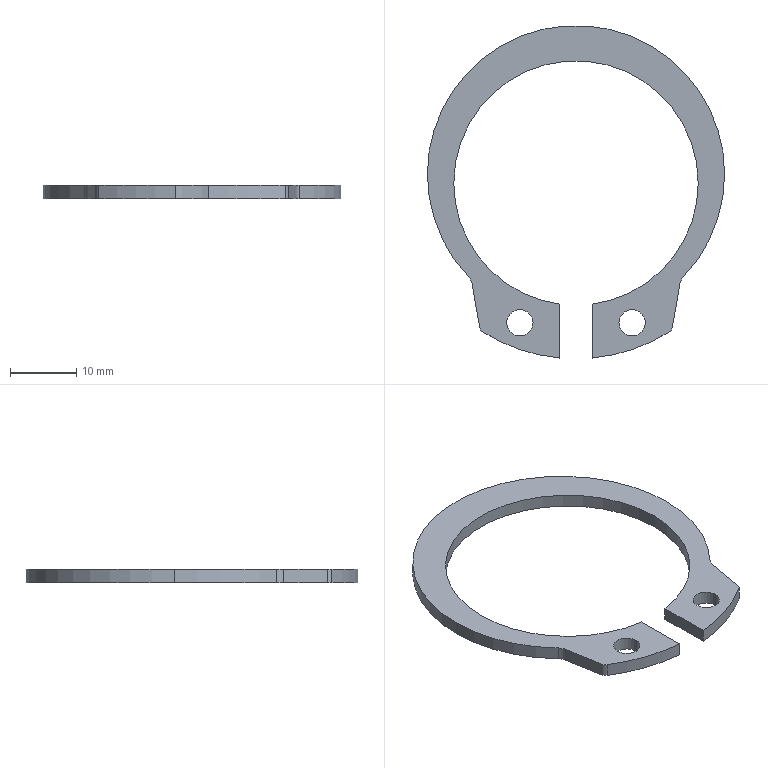Part | SolidWorks | features Extrusion 1 | 1 solid | 22 faces | box 45 x 50.322 x 2 mm | volume 1249 mm3 | cylinder 16 | plane 6 | commonest cylinder face diameters 4 x6 37 x3 45 x3 2 x2 53.2 x2
STEP:
#1=CARTESIAN_POINT('',(6.5,-22.5,2.));
#2=VERTEX_POINT('',#1);
#3=CARTESIAN_POINT('',(10.5,-22.5,2.));
#4=VERTEX_POINT('',#3);
#5=CARTESIAN_POINT('',(8.5,-22.5,2.));
#6=DIRECTION('',(0.,0.,1.));
#7=DIRECTION('',(1.,0.,0.));
#8=AXIS2_PLACEMENT_3D('',#5,#6,#7);
#9=CIRCLE('',#8,2.);
#10=EDGE_CURVE('',#2,#4,#9,.T.);
#11=ORIENTED_EDGE('',*,*,#10,.T.);
#12=CARTESIAN_POINT('',(10.5,-22.5,0.));
#13=VERTEX_POINT('',#12);
#14=CARTESIAN_POINT('',(10.5,-22.5,2.));
#15=DIRECTION('',(0.,0.,-1.));
#16=VECTOR('',#15,1000.);
#17=LINE('',#14,#16);
#18=EDGE_CURVE('',#4,#13,#17,.T.);
#19=ORIENTED_EDGE('',*,*,#18,.T.);
#20=CARTESIAN_POINT('',(6.5,-22.5,0.));
#21=VERTEX_POINT('',#20);
#22=CARTESIAN_POINT('',(8.5,-22.5,0.));
#23=DIRECTION('',(0.,0.,1.));
#24=DIRECTION('',(1.,0.,0.));
#25=AXIS2_PLACEMENT_3D('',#22,#23,#24);
#26=CIRCLE('',#25,2.);
#27=EDGE_CURVE('',#21,#13,#26,.T.);
#28=ORIENTED_EDGE('',*,*,#27,.F.);
#29=CARTESIAN_POINT('',(6.5,-22.5,2.));
#30=DIRECTION('',(0.,0.,-1.));
#31=VECTOR('',#30,1000.);
#32=LINE('',#29,#31);
#33=EDGE_CURVE('',#2,#21,#32,.T.);
#34=ORIENTED_EDGE('',*,*,#33,.F.);
#35=EDGE_LOOP('',(#11,#19,#28,#34));
#36=FACE_OUTER_BOUND('',#35,.T.);
#37=CARTESIAN_POINT('',(8.5,-22.5,2.));
#38=DIRECTION('',(0.,0.,-1.));
#39=DIRECTION('',(-1.,0.,0.));
#40=AXIS2_PLACEMENT_3D('',#37,#38,#39);
#41=CYLINDRICAL_SURFACE('',#40,2.);
#42=ADVANCED_FACE('',(#36),#41,.F.);
#43=CARTESIAN_POINT('',(-10.5,-22.5,2.));
#44=VERTEX_POINT('',#43);
#45=CARTESIAN_POINT('',(-6.5,-22.5,2.));
#46=VERTEX_POINT('',#45);
#47=CARTESIAN_POINT('',(-8.5,-22.5,2.));
#48=DIRECTION('',(0.,0.,1.));
#49=DIRECTION('',(1.,0.,0.));
#50=AXIS2_PLACEMENT_3D('',#47,#48,#49);
#51=CIRCLE('',#50,2.);
#52=EDGE_CURVE('',#44,#46,#51,.T.);
#53=ORIENTED_EDGE('',*,*,#52,.T.);
#54=CARTESIAN_POINT('',(-6.5,-22.5,0.));
#55=VERTEX_POINT('',#54);
#56=CARTESIAN_POINT('',(-6.5,-22.5,2.));
#57=DIRECTION('',(0.,0.,-1.));
#58=VECTOR('',#57,1000.);
#59=LINE('',#56,#58);
#60=EDGE_CURVE('',#46,#55,#59,.T.);
#61=ORIENTED_EDGE('',*,*,#60,.T.);
#62=CARTESIAN_POINT('',(-10.5,-22.5,0.));
#63=VERTEX_POINT('',#62);
#64=CARTESIAN_POINT('',(-8.5,-22.5,0.));
#65=DIRECTION('',(0.,0.,1.));
#66=DIRECTION('',(1.,0.,0.));
#67=AXIS2_PLACEMENT_3D('',#64,#65,#66);
#68=CIRCLE('',#67,2.);
#69=EDGE_CURVE('',#63,#55,#68,.T.);
#70=ORIENTED_EDGE('',*,*,#69,.F.);
#71=CARTESIAN_POINT('',(-10.5,-22.5,2.));
#72=DIRECTION('',(0.,0.,-1.));
#73=VECTOR('',#72,1000.);
#74=LINE('',#71,#73);
#75=EDGE_CURVE('',#44,#63,#74,.T.);
#76=ORIENTED_EDGE('',*,*,#75,.F.);
#77=EDGE_LOOP('',(#53,#61,#70,#76));
#78=FACE_OUTER_BOUND('',#77,.T.);
#79=CARTESIAN_POINT('',(-8.5,-22.5,2.));
#80=DIRECTION('',(0.,0.,-1.));
#81=DIRECTION('',(-1.,0.,0.));
#82=AXIS2_PLACEMENT_3D('',#79,#80,#81);
#83=CYLINDRICAL_SURFACE('',#82,2.);
#84=ADVANCED_FACE('',(#78),#83,.F.);
#85=CARTESIAN_POINT('',(22.5,0.,2.));
#86=VERTEX_POINT('',#85);
#87=CARTESIAN_POINT('',(-22.5,0.,2.));
#88=VERTEX_POINT('',#87);
#89=CARTESIAN_POINT('',(0.,0.,2.));
#90=DIRECTION('',(0.,0.,1.));
#91=DIRECTION('',(1.,0.,0.));
#92=AXIS2_PLACEMENT_3D('',#89,#90,#91);
#93=CIRCLE('',#92,22.5);
#94=EDGE_CURVE('',#86,#88,#93,.T.);
#95=ORIENTED_EDGE('',*,*,#94,.F.);
#96=CARTESIAN_POINT('',(22.5,0.,0.));
#97=VERTEX_POINT('',#96);
#98=CARTESIAN_POINT('',(22.5,0.,2.));
#99=DIRECTION('',(0.,0.,-1.));
#100=VECTOR('',#99,1000.);
#101=LINE('',#98,#100);
#102=EDGE_CURVE('',#86,#97,#101,.T.);
#103=ORIENTED_EDGE('',*,*,#102,.T.);
#104=CARTESIAN_POINT('',(-22.5,0.,0.));
#105=VERTEX_POINT('',#104);
#106=CARTESIAN_POINT('',(0.,0.,0.));
#107=DIRECTION('',(0.,0.,1.));
#108=DIRECTION('',(1.,0.,0.));
#109=AXIS2_PLACEMENT_3D('',#106,#107,#108);
#110=CIRCLE('',#109,22.5);
#111=EDGE_CURVE('',#97,#105,#110,.T.);
#112=ORIENTED_EDGE('',*,*,#111,.T.);
#113=CARTESIAN_POINT('',(-22.5,0.,2.));
#114=DIRECTION('',(0.,0.,-1.));
#115=VECTOR('',#114,1000.);
#116=LINE('',#113,#115);
#117=EDGE_CURVE('',#88,#105,#116,.T.);
#118=ORIENTED_EDGE('',*,*,#117,.F.);
#119=EDGE_LOOP('',(#95,#103,#112,#118));
#120=FACE_OUTER_BOUND('',#119,.T.);
#121=CARTESIAN_POINT('',(0.,0.,2.));
#122=DIRECTION('',(0.,0.,-1.));
#123=DIRECTION('',(-1.,0.,0.));
#124=AXIS2_PLACEMENT_3D('',#121,#122,#123);
#125=CYLINDRICAL_SURFACE('',#124,22.5);
#126=ADVANCED_FACE('',(#120),#125,.T.);
#127=CARTESIAN_POINT('',(-16.266,-15.545,2.));
#128=VERTEX_POINT('',#127);
#129=CARTESIAN_POINT('',(0.,0.,2.));
#130=DIRECTION('',(0.,0.,1.));
#131=DIRECTION('',(1.,0.,0.));
#132=AXIS2_PLACEMENT_3D('',#129,#130,#131);
#133=CIRCLE('',#132,22.5);
#134=EDGE_CURVE('',#88,#128,#133,.T.);
#135=ORIENTED_EDGE('',*,*,#134,.F.);
#136=ORIENTED_EDGE('',*,*,#117,.T.);
#137=CARTESIAN_POINT('',(-16.266,-15.545,0.));
#138=VERTEX_POINT('',#137);
#139=CARTESIAN_POINT('',(0.,0.,0.));
#140=DIRECTION('',(0.,0.,1.));
#141=DIRECTION('',(1.,0.,0.));
#142=AXIS2_PLACEMENT_3D('',#139,#140,#141);
#143=CIRCLE('',#142,22.5);
#144=EDGE_CURVE('',#105,#138,#143,.T.);
#145=ORIENTED_EDGE('',*,*,#144,.T.);
#146=CARTESIAN_POINT('',(-16.266,-15.545,2.));
#147=DIRECTION('',(0.,0.,-1.));
#148=VECTOR('',#147,1000.);
#149=LINE('',#146,#148);
#150=EDGE_CURVE('',#128,#138,#149,.T.);
#151=ORIENTED_EDGE('',*,*,#150,.F.);
#152=EDGE_LOOP('',(#135,#136,#145,#151));
#153=FACE_OUTER_BOUND('',#152,.T.);
#154=CARTESIAN_POINT('',(0.,0.,2.));
#155=DIRECTION('',(0.,0.,-1.));
#156=DIRECTION('',(-1.,0.,0.));
#157=AXIS2_PLACEMENT_3D('',#154,#155,#156);
#158=CYLINDRICAL_SURFACE('',#157,22.5);
#159=ADVANCED_FACE('',(#153),#158,.T.);
#160=CARTESIAN_POINT('',(18.5,-1.34,2.));
#161=VERTEX_POINT('',#160);
#162=CARTESIAN_POINT('',(2.5,-19.67,2.));
#163=VERTEX_POINT('',#162);
#164=CARTESIAN_POINT('',(0.,-1.34,2.));
#165=DIRECTION('',(0.,0.,-1.));
#166=DIRECTION('',(1.,0.,0.));
#167=AXIS2_PLACEMENT_3D('',#164,#165,#166);
#168=CIRCLE('',#167,18.5);
#169=EDGE_CURVE('',#161,#163,#168,.T.);
#170=ORIENTED_EDGE('',*,*,#169,.F.);
#171=CARTESIAN_POINT('',(18.5,-1.34,0.));
#172=VERTEX_POINT('',#171);
#173=CARTESIAN_POINT('',(18.5,-1.34,2.));
#174=DIRECTION('',(0.,0.,-1.));
#175=VECTOR('',#174,1000.);
#176=LINE('',#173,#175);
#177=EDGE_CURVE('',#161,#172,#176,.T.);
#178=ORIENTED_EDGE('',*,*,#177,.T.);
#179=CARTESIAN_POINT('',(2.5,-19.67,0.));
#180=VERTEX_POINT('',#179);
#181=CARTESIAN_POINT('',(0.,-1.34,0.));
#182=DIRECTION('',(0.,0.,-1.));
#183=DIRECTION('',(1.,0.,0.));
#184=AXIS2_PLACEMENT_3D('',#181,#182,#183);
#185=CIRCLE('',#184,18.5);
#186=EDGE_CURVE('',#172,#180,#185,.T.);
#187=ORIENTED_EDGE('',*,*,#186,.T.);
#188=CARTESIAN_POINT('',(2.5,-19.67,2.));
#189=DIRECTION('',(0.,0.,-1.));
#190=VECTOR('',#189,1000.);
#191=LINE('',#188,#190);
#192=EDGE_CURVE('',#163,#180,#191,.T.);
#193=ORIENTED_EDGE('',*,*,#192,.F.);
#194=EDGE_LOOP('',(#170,#178,#187,#193));
#195=FACE_OUTER_BOUND('',#194,.T.);
#196=CARTESIAN_POINT('',(0.,-1.34,2.));
#197=DIRECTION('',(0.,0.,-1.));
#198=DIRECTION('',(-1.,0.,0.));
#199=AXIS2_PLACEMENT_3D('',#196,#197,#198);
#200=CYLINDRICAL_SURFACE('',#199,18.5);
#201=ADVANCED_FACE('',(#195),#200,.F.);
#202=ORIENTED_EDGE('',*,*,#177,.F.);
#203=CARTESIAN_POINT('',(-18.5,-1.34,2.));
#204=VERTEX_POINT('',#203);
#205=CARTESIAN_POINT('',(0.,-1.34,2.));
#206=DIRECTION('',(0.,0.,-1.));
#207=DIRECTION('',(1.,0.,0.));
#208=AXIS2_PLACEMENT_3D('',#205,#206,#207);
#209=CIRCLE('',#208,18.5);
#210=EDGE_CURVE('',#204,#161,#209,.T.);
#211=ORIENTED_EDGE('',*,*,#210,.F.);
#212=CARTESIAN_POINT('',(-18.5,-1.34,0.));
#213=VERTEX_POINT('',#212);
#214=CARTESIAN_POINT('',(-18.5,-1.34,2.));
#215=DIRECTION('',(0.,0.,-1.));
#216=VECTOR('',#215,1000.);
#217=LINE('',#214,#216);
#218=EDGE_CURVE('',#204,#213,#217,.T.);
#219=ORIENTED_EDGE('',*,*,#218,.T.);
#220=CARTESIAN_POINT('',(0.,-1.34,0.));
#221=DIRECTION('',(0.,0.,-1.));
#222=DIRECTION('',(1.,0.,0.));
#223=AXIS2_PLACEMENT_3D('',#220,#221,#222);
#224=CIRCLE('',#223,18.5);
#225=EDGE_CURVE('',#213,#172,#224,.T.);
#226=ORIENTED_EDGE('',*,*,#225,.T.);
#227=EDGE_LOOP('',(#202,#211,#219,#226));
#228=FACE_OUTER_BOUND('',#227,.T.);
#229=CARTESIAN_POINT('',(0.,-1.34,2.));
#230=DIRECTION('',(0.,0.,-1.));
#231=DIRECTION('',(-1.,0.,0.));
#232=AXIS2_PLACEMENT_3D('',#229,#230,#231);
#233=CYLINDRICAL_SURFACE('',#232,18.5);
#234=ADVANCED_FACE('',(#228),#233,.F.);
#235=ORIENTED_EDGE('',*,*,#52,.F.);
#236=CARTESIAN_POINT('',(-8.5,-22.5,2.));
#237=DIRECTION('',(0.,0.,1.));
#238=DIRECTION('',(1.,0.,0.));
#239=AXIS2_PLACEMENT_3D('',#236,#237,#238);
#240=CIRCLE('',#239,2.);
#241=EDGE_CURVE('',#46,#44,#240,.T.);
#242=ORIENTED_EDGE('',*,*,#241,.F.);
#243=EDGE_LOOP('',(#235,#242));
#244=FACE_BOUND('',#243,.T.);
#245=CARTESIAN_POINT('',(-14.122,-23.882,2.));
#246=VERTEX_POINT('',#245);
#247=CARTESIAN_POINT('',(-2.5,-27.822,2.));
#248=VERTEX_POINT('',#247);
#249=CARTESIAN_POINT('',(0.,-1.34,2.));
#250=DIRECTION('',(0.,0.,1.));
#251=DIRECTION('',(1.,0.,0.));
#252=AXIS2_PLACEMENT_3D('',#249,#250,#251);
#253=CIRCLE('',#252,26.6);
#254=EDGE_CURVE('',#246,#248,#253,.T.);
#255=ORIENTED_EDGE('',*,*,#254,.T.);
#256=CARTESIAN_POINT('',(-2.5,-19.67,2.));
#257=VERTEX_POINT('',#256);
#258=CARTESIAN_POINT('',(-2.5,-27.822,2.));
#259=DIRECTION('',(0.,1.,0.));
#260=VECTOR('',#259,1000.);
#261=LINE('',#258,#260);
#262=EDGE_CURVE('',#248,#257,#261,.T.);
#263=ORIENTED_EDGE('',*,*,#262,.T.);
#264=CARTESIAN_POINT('',(0.,-1.34,2.));
#265=DIRECTION('',(0.,0.,-1.));
#266=DIRECTION('',(1.,0.,0.));
#267=AXIS2_PLACEMENT_3D('',#264,#265,#266);
#268=CIRCLE('',#267,18.5);
#269=EDGE_CURVE('',#257,#204,#268,.T.);
#270=ORIENTED_EDGE('',*,*,#269,.T.);
#271=ORIENTED_EDGE('',*,*,#210,.T.);
#272=ORIENTED_EDGE('',*,*,#169,.T.);
#273=CARTESIAN_POINT('',(2.5,-27.822,2.));
#274=VERTEX_POINT('',#273);
#275=CARTESIAN_POINT('',(2.5,-27.822,2.));
#276=DIRECTION('',(0.,-1.,0.));
#277=VECTOR('',#276,1000.);
#278=LINE('',#275,#277);
#279=EDGE_CURVE('',#163,#274,#278,.T.);
#280=ORIENTED_EDGE('',*,*,#279,.T.);
#281=CARTESIAN_POINT('',(14.122,-23.882,2.));
#282=VERTEX_POINT('',#281);
#283=CARTESIAN_POINT('',(0.,-1.34,2.));
#284=DIRECTION('',(0.,0.,1.));
#285=DIRECTION('',(1.,0.,0.));
#286=AXIS2_PLACEMENT_3D('',#283,#284,#285);
#287=CIRCLE('',#286,26.6);
#288=EDGE_CURVE('',#274,#282,#287,.T.);
#289=ORIENTED_EDGE('',*,*,#288,.T.);
#290=CARTESIAN_POINT('',(14.576,-23.207,2.));
#291=VERTEX_POINT('',#290);
#292=CARTESIAN_POINT('',(13.591,-23.034,2.));
#293=DIRECTION('',(0.,0.,1.));
#294=DIRECTION('',(-1.,0.,0.));
#295=AXIS2_PLACEMENT_3D('',#292,#293,#294);
#296=CIRCLE('',#295,1.);
#297=EDGE_CURVE('',#282,#291,#296,.T.);
#298=ORIENTED_EDGE('',*,*,#297,.T.);
#299=CARTESIAN_POINT('',(15.742,-16.58,2.));
#300=VERTEX_POINT('',#299);
#301=CARTESIAN_POINT('',(14.576,-23.207,2.));
#302=DIRECTION('',(0.1733,0.9849,0.));
#303=VECTOR('',#302,1000.);
#304=LINE('',#301,#303);
#305=EDGE_CURVE('',#291,#300,#304,.T.);
#306=ORIENTED_EDGE('',*,*,#305,.T.);
#307=CARTESIAN_POINT('',(16.266,-15.545,2.));
#308=VERTEX_POINT('',#307);
#309=CARTESIAN_POINT('',(17.712,-16.927,2.));
#310=DIRECTION('',(0.,0.,-1.));
#311=DIRECTION('',(-1.,0.,0.));
#312=AXIS2_PLACEMENT_3D('',#309,#310,#311);
#313=CIRCLE('',#312,2.);
#314=EDGE_CURVE('',#300,#308,#313,.T.);
#315=ORIENTED_EDGE('',*,*,#314,.T.);
#316=CARTESIAN_POINT('',(0.,0.,2.));
#317=DIRECTION('',(0.,0.,1.));
#318=DIRECTION('',(1.,0.,0.));
#319=AXIS2_PLACEMENT_3D('',#316,#317,#318);
#320=CIRCLE('',#319,22.5);
#321=EDGE_CURVE('',#308,#86,#320,.T.);
#322=ORIENTED_EDGE('',*,*,#321,.T.);
#323=ORIENTED_EDGE('',*,*,#94,.T.);
#324=ORIENTED_EDGE('',*,*,#134,.T.);
#325=CARTESIAN_POINT('',(-15.742,-16.58,2.));
#326=VERTEX_POINT('',#325);
#327=CARTESIAN_POINT('',(-17.712,-16.927,2.));
#328=DIRECTION('',(0.,0.,-1.));
#329=DIRECTION('',(1.,0.,0.));
#330=AXIS2_PLACEMENT_3D('',#327,#328,#329);
#331=CIRCLE('',#330,2.);
#332=EDGE_CURVE('',#128,#326,#331,.T.);
#333=ORIENTED_EDGE('',*,*,#332,.T.);
#334=CARTESIAN_POINT('',(-14.576,-23.207,2.));
#335=VERTEX_POINT('',#334);
#336=CARTESIAN_POINT('',(-14.576,-23.207,2.));
#337=DIRECTION('',(0.1733,-0.9849,0.));
#338=VECTOR('',#337,1000.);
#339=LINE('',#336,#338);
#340=EDGE_CURVE('',#326,#335,#339,.T.);
#341=ORIENTED_EDGE('',*,*,#340,.T.);
#342=CARTESIAN_POINT('',(-13.591,-23.034,2.));
#343=DIRECTION('',(0.,0.,1.));
#344=DIRECTION('',(-1.,0.,0.));
#345=AXIS2_PLACEMENT_3D('',#342,#343,#344);
#346=CIRCLE('',#345,1.);
#347=EDGE_CURVE('',#335,#246,#346,.T.);
#348=ORIENTED_EDGE('',*,*,#347,.T.);
#349=EDGE_LOOP('',(#255,#263,#270,#271,#272,#280,#289,#298,#306,#315,#322,#323,#324,#333,#341,#348));
#350=FACE_OUTER_BOUND('',#349,.T.);
#351=ORIENTED_EDGE('',*,*,#10,.F.);
#352=CARTESIAN_POINT('',(8.5,-22.5,2.));
#353=DIRECTION('',(0.,0.,1.));
#354=DIRECTION('',(1.,0.,0.));
#355=AXIS2_PLACEMENT_3D('',#352,#353,#354);
#356=CIRCLE('',#355,2.);
#357=EDGE_CURVE('',#4,#2,#356,.T.);
#358=ORIENTED_EDGE('',*,*,#357,.F.);
#359=EDGE_LOOP('',(#351,#358));
#360=FACE_BOUND('',#359,.T.);
#361=CARTESIAN_POINT('',(0.,-1.34,2.));
#362=DIRECTION('',(0.,0.,1.));
#363=DIRECTION('',(1.,0.,0.));
#364=AXIS2_PLACEMENT_3D('',#361,#362,#363);
#365=PLANE('',#364);
#366=ADVANCED_FACE('',(#244,#350,#360),#365,.T.);
#367=CARTESIAN_POINT('',(-14.122,-23.882,0.));
#368=VERTEX_POINT('',#367);
#369=CARTESIAN_POINT('',(-2.5,-27.822,0.));
#370=VERTEX_POINT('',#369);
#371=CARTESIAN_POINT('',(0.,-1.34,0.));
#372=DIRECTION('',(0.,0.,1.));
#373=DIRECTION('',(1.,0.,0.));
#374=AXIS2_PLACEMENT_3D('',#371,#372,#373);
#375=CIRCLE('',#374,26.6);
#376=EDGE_CURVE('',#368,#370,#375,.T.);
#377=ORIENTED_EDGE('',*,*,#376,.F.);
#378=CARTESIAN_POINT('',(-14.576,-23.207,0.));
#379=VERTEX_POINT('',#378);
#380=CARTESIAN_POINT('',(-13.591,-23.034,0.));
#381=DIRECTION('',(0.,0.,1.));
#382=DIRECTION('',(-1.,0.,0.));
#383=AXIS2_PLACEMENT_3D('',#380,#381,#382);
#384=CIRCLE('',#383,1.);
#385=EDGE_CURVE('',#379,#368,#384,.T.);
#386=ORIENTED_EDGE('',*,*,#385,.F.);
#387=CARTESIAN_POINT('',(-15.742,-16.58,0.));
#388=VERTEX_POINT('',#387);
#389=CARTESIAN_POINT('',(-14.576,-23.207,0.));
#390=DIRECTION('',(0.1733,-0.9849,0.));
#391=VECTOR('',#390,1000.);
#392=LINE('',#389,#391);
#393=EDGE_CURVE('',#388,#379,#392,.T.);
#394=ORIENTED_EDGE('',*,*,#393,.F.);
#395=CARTESIAN_POINT('',(-17.712,-16.927,0.));
#396=DIRECTION('',(0.,0.,-1.));
#397=DIRECTION('',(1.,0.,0.));
#398=AXIS2_PLACEMENT_3D('',#395,#396,#397);
#399=CIRCLE('',#398,2.);
#400=EDGE_CURVE('',#138,#388,#399,.T.);
#401=ORIENTED_EDGE('',*,*,#400,.F.);
#402=ORIENTED_EDGE('',*,*,#144,.F.);
#403=ORIENTED_EDGE('',*,*,#111,.F.);
#404=CARTESIAN_POINT('',(16.266,-15.545,0.));
#405=VERTEX_POINT('',#404);
#406=CARTESIAN_POINT('',(0.,0.,0.));
#407=DIRECTION('',(0.,0.,1.));
#408=DIRECTION('',(1.,0.,0.));
#409=AXIS2_PLACEMENT_3D('',#406,#407,#408);
#410=CIRCLE('',#409,22.5);
#411=EDGE_CURVE('',#405,#97,#410,.T.);
#412=ORIENTED_EDGE('',*,*,#411,.F.);
#413=CARTESIAN_POINT('',(15.742,-16.58,0.));
#414=VERTEX_POINT('',#413);
#415=CARTESIAN_POINT('',(17.712,-16.927,0.));
#416=DIRECTION('',(0.,0.,-1.));
#417=DIRECTION('',(-1.,0.,0.));
#418=AXIS2_PLACEMENT_3D('',#415,#416,#417);
#419=CIRCLE('',#418,2.);
#420=EDGE_CURVE('',#414,#405,#419,.T.);
#421=ORIENTED_EDGE('',*,*,#420,.F.);
#422=CARTESIAN_POINT('',(14.576,-23.207,0.));
#423=VERTEX_POINT('',#422);
#424=CARTESIAN_POINT('',(14.576,-23.207,0.));
#425=DIRECTION('',(0.1733,0.9849,0.));
#426=VECTOR('',#425,1000.);
#427=LINE('',#424,#426);
#428=EDGE_CURVE('',#423,#414,#427,.T.);
#429=ORIENTED_EDGE('',*,*,#428,.F.);
#430=CARTESIAN_POINT('',(14.122,-23.882,0.));
#431=VERTEX_POINT('',#430);
#432=CARTESIAN_POINT('',(13.591,-23.034,0.));
#433=DIRECTION('',(0.,0.,1.));
#434=DIRECTION('',(-1.,0.,0.));
#435=AXIS2_PLACEMENT_3D('',#432,#433,#434);
#436=CIRCLE('',#435,1.);
#437=EDGE_CURVE('',#431,#423,#436,.T.);
#438=ORIENTED_EDGE('',*,*,#437,.F.);
#439=CARTESIAN_POINT('',(2.5,-27.822,0.));
#440=VERTEX_POINT('',#439);
#441=CARTESIAN_POINT('',(0.,-1.34,0.));
#442=DIRECTION('',(0.,0.,1.));
#443=DIRECTION('',(1.,0.,0.));
#444=AXIS2_PLACEMENT_3D('',#441,#442,#443);
#445=CIRCLE('',#444,26.6);
#446=EDGE_CURVE('',#440,#431,#445,.T.);
#447=ORIENTED_EDGE('',*,*,#446,.F.);
#448=CARTESIAN_POINT('',(2.5,-27.822,0.));
#449=DIRECTION('',(0.,-1.,0.));
#450=VECTOR('',#449,1000.);
#451=LINE('',#448,#450);
#452=EDGE_CURVE('',#180,#440,#451,.T.);
#453=ORIENTED_EDGE('',*,*,#452,.F.);
#454=ORIENTED_EDGE('',*,*,#186,.F.);
#455=ORIENTED_EDGE('',*,*,#225,.F.);
#456=CARTESIAN_POINT('',(-2.5,-19.67,0.));
#457=VERTEX_POINT('',#456);
#458=CARTESIAN_POINT('',(0.,-1.34,0.));
#459=DIRECTION('',(0.,0.,-1.));
#460=DIRECTION('',(1.,0.,0.));
#461=AXIS2_PLACEMENT_3D('',#458,#459,#460);
#462=CIRCLE('',#461,18.5);
#463=EDGE_CURVE('',#457,#213,#462,.T.);
#464=ORIENTED_EDGE('',*,*,#463,.F.);
#465=CARTESIAN_POINT('',(-2.5,-27.822,0.));
#466=DIRECTION('',(0.,1.,0.));
#467=VECTOR('',#466,1000.);
#468=LINE('',#465,#467);
#469=EDGE_CURVE('',#370,#457,#468,.T.);
#470=ORIENTED_EDGE('',*,*,#469,.F.);
#471=EDGE_LOOP('',(#377,#386,#394,#401,#402,#403,#412,#421,#429,#438,#447,#453,#454,#455,#464,#470));
#472=FACE_OUTER_BOUND('',#471,.T.);
#473=ORIENTED_EDGE('',*,*,#69,.T.);
#474=CARTESIAN_POINT('',(-8.5,-22.5,0.));
#475=DIRECTION('',(0.,0.,1.));
#476=DIRECTION('',(1.,0.,0.));
#477=AXIS2_PLACEMENT_3D('',#474,#475,#476);
#478=CIRCLE('',#477,2.);
#479=EDGE_CURVE('',#55,#63,#478,.T.);
#480=ORIENTED_EDGE('',*,*,#479,.T.);
#481=EDGE_LOOP('',(#473,#480));
#482=FACE_BOUND('',#481,.T.);
#483=ORIENTED_EDGE('',*,*,#27,.T.);
#484=CARTESIAN_POINT('',(8.5,-22.5,0.));
#485=DIRECTION('',(0.,0.,1.));
#486=DIRECTION('',(1.,0.,0.));
#487=AXIS2_PLACEMENT_3D('',#484,#485,#486);
#488=CIRCLE('',#487,2.);
#489=EDGE_CURVE('',#13,#21,#488,.T.);
#490=ORIENTED_EDGE('',*,*,#489,.T.);
#491=EDGE_LOOP('',(#483,#490));
#492=FACE_BOUND('',#491,.T.);
#493=CARTESIAN_POINT('',(0.,-1.34,0.));
#494=DIRECTION('',(0.,0.,1.));
#495=DIRECTION('',(1.,0.,0.));
#496=AXIS2_PLACEMENT_3D('',#493,#494,#495);
#497=PLANE('',#496);
#498=ADVANCED_FACE('',(#472,#482,#492),#497,.F.);
#499=ORIENTED_EDGE('',*,*,#376,.T.);
#500=CARTESIAN_POINT('',(-2.5,-27.822,2.));
#501=DIRECTION('',(0.,0.,-1.));
#502=VECTOR('',#501,1000.);
#503=LINE('',#500,#502);
#504=EDGE_CURVE('',#248,#370,#503,.T.);
#505=ORIENTED_EDGE('',*,*,#504,.F.);
#506=ORIENTED_EDGE('',*,*,#254,.F.);
#507=CARTESIAN_POINT('',(-14.122,-23.882,2.));
#508=DIRECTION('',(0.,0.,-1.));
#509=VECTOR('',#508,1000.);
#510=LINE('',#507,#509);
#511=EDGE_CURVE('',#246,#368,#510,.T.);
#512=ORIENTED_EDGE('',*,*,#511,.T.);
#513=EDGE_LOOP('',(#499,#505,#506,#512));
#514=FACE_OUTER_BOUND('',#513,.T.);
#515=CARTESIAN_POINT('',(0.,-1.34,2.));
#516=DIRECTION('',(0.,0.,-1.));
#517=DIRECTION('',(-1.,0.,0.));
#518=AXIS2_PLACEMENT_3D('',#515,#516,#517);
#519=CYLINDRICAL_SURFACE('',#518,26.6);
#520=ADVANCED_FACE('',(#514),#519,.T.);
#521=ORIENTED_EDGE('',*,*,#469,.T.);
#522=CARTESIAN_POINT('',(-2.5,-19.67,2.));
#523=DIRECTION('',(0.,0.,-1.));
#524=VECTOR('',#523,1000.);
#525=LINE('',#522,#524);
#526=EDGE_CURVE('',#257,#457,#525,.T.);
#527=ORIENTED_EDGE('',*,*,#526,.F.);
#528=ORIENTED_EDGE('',*,*,#262,.F.);
#529=ORIENTED_EDGE('',*,*,#504,.T.);
#530=EDGE_LOOP('',(#521,#527,#528,#529));
#531=FACE_OUTER_BOUND('',#530,.T.);
#532=CARTESIAN_POINT('',(-2.5,-27.822,2.));
#533=DIRECTION('',(-1.,0.,0.));
#534=DIRECTION('',(0.,0.,1.));
#535=AXIS2_PLACEMENT_3D('',#532,#533,#534);
#536=PLANE('',#535);
#537=ADVANCED_FACE('',(#531),#536,.F.);
#538=ORIENTED_EDGE('',*,*,#218,.F.);
#539=ORIENTED_EDGE('',*,*,#269,.F.);
#540=ORIENTED_EDGE('',*,*,#526,.T.);
#541=ORIENTED_EDGE('',*,*,#463,.T.);
#542=EDGE_LOOP('',(#538,#539,#540,#541));
#543=FACE_OUTER_BOUND('',#542,.T.);
#544=CARTESIAN_POINT('',(0.,-1.34,2.));
#545=DIRECTION('',(0.,0.,-1.));
#546=DIRECTION('',(-1.,0.,0.));
#547=AXIS2_PLACEMENT_3D('',#544,#545,#546);
#548=CYLINDRICAL_SURFACE('',#547,18.5);
#549=ADVANCED_FACE('',(#543),#548,.F.);
#550=ORIENTED_EDGE('',*,*,#452,.T.);
#551=CARTESIAN_POINT('',(2.5,-27.822,2.));
#552=DIRECTION('',(0.,0.,-1.));
#553=VECTOR('',#552,1000.);
#554=LINE('',#551,#553);
#555=EDGE_CURVE('',#274,#440,#554,.T.);
#556=ORIENTED_EDGE('',*,*,#555,.F.);
#557=ORIENTED_EDGE('',*,*,#279,.F.);
#558=ORIENTED_EDGE('',*,*,#192,.T.);
#559=EDGE_LOOP('',(#550,#556,#557,#558));
#560=FACE_OUTER_BOUND('',#559,.T.);
#561=CARTESIAN_POINT('',(2.5,-27.822,2.));
#562=DIRECTION('',(1.,0.,0.));
#563=DIRECTION('',(0.,0.,-1.));
#564=AXIS2_PLACEMENT_3D('',#561,#562,#563);
#565=PLANE('',#564);
#566=ADVANCED_FACE('',(#560),#565,.F.);
#567=ORIENTED_EDGE('',*,*,#446,.T.);
#568=CARTESIAN_POINT('',(14.122,-23.882,2.));
#569=DIRECTION('',(0.,0.,-1.));
#570=VECTOR('',#569,1000.);
#571=LINE('',#568,#570);
#572=EDGE_CURVE('',#282,#431,#571,.T.);
#573=ORIENTED_EDGE('',*,*,#572,.F.);
#574=ORIENTED_EDGE('',*,*,#288,.F.);
#575=ORIENTED_EDGE('',*,*,#555,.T.);
#576=EDGE_LOOP('',(#567,#573,#574,#575));
#577=FACE_OUTER_BOUND('',#576,.T.);
#578=CARTESIAN_POINT('',(0.,-1.34,2.));
#579=DIRECTION('',(0.,0.,-1.));
#580=DIRECTION('',(-1.,0.,0.));
#581=AXIS2_PLACEMENT_3D('',#578,#579,#580);
#582=CYLINDRICAL_SURFACE('',#581,26.6);
#583=ADVANCED_FACE('',(#577),#582,.T.);
#584=ORIENTED_EDGE('',*,*,#437,.T.);
#585=CARTESIAN_POINT('',(14.576,-23.207,2.));
#586=DIRECTION('',(0.,0.,-1.));
#587=VECTOR('',#586,1000.);
#588=LINE('',#585,#587);
#589=EDGE_CURVE('',#291,#423,#588,.T.);
#590=ORIENTED_EDGE('',*,*,#589,.F.);
#591=ORIENTED_EDGE('',*,*,#297,.F.);
#592=ORIENTED_EDGE('',*,*,#572,.T.);
#593=EDGE_LOOP('',(#584,#590,#591,#592));
#594=FACE_OUTER_BOUND('',#593,.T.);
#595=CARTESIAN_POINT('',(13.591,-23.034,2.));
#596=DIRECTION('',(0.,0.,-1.));
#597=DIRECTION('',(-1.,0.,0.));
#598=AXIS2_PLACEMENT_3D('',#595,#596,#597);
#599=CYLINDRICAL_SURFACE('',#598,1.);
#600=ADVANCED_FACE('',(#594),#599,.T.);
#601=ORIENTED_EDGE('',*,*,#428,.T.);
#602=CARTESIAN_POINT('',(15.742,-16.58,2.));
#603=DIRECTION('',(0.,0.,-1.));
#604=VECTOR('',#603,1000.);
#605=LINE('',#602,#604);
#606=EDGE_CURVE('',#300,#414,#605,.T.);
#607=ORIENTED_EDGE('',*,*,#606,.F.);
#608=ORIENTED_EDGE('',*,*,#305,.F.);
#609=ORIENTED_EDGE('',*,*,#589,.T.);
#610=EDGE_LOOP('',(#601,#607,#608,#609));
#611=FACE_OUTER_BOUND('',#610,.T.);
#612=CARTESIAN_POINT('',(14.576,-23.207,2.));
#613=DIRECTION('',(-0.9849,0.1733,0.));
#614=DIRECTION('',(-0.1733,-0.9849,0.));
#615=AXIS2_PLACEMENT_3D('',#612,#613,#614);
#616=PLANE('',#615);
#617=ADVANCED_FACE('',(#611),#616,.F.);
#618=ORIENTED_EDGE('',*,*,#420,.T.);
#619=CARTESIAN_POINT('',(16.266,-15.545,2.));
#620=DIRECTION('',(0.,0.,-1.));
#621=VECTOR('',#620,1000.);
#622=LINE('',#619,#621);
#623=EDGE_CURVE('',#308,#405,#622,.T.);
#624=ORIENTED_EDGE('',*,*,#623,.F.);
#625=ORIENTED_EDGE('',*,*,#314,.F.);
#626=ORIENTED_EDGE('',*,*,#606,.T.);
#627=EDGE_LOOP('',(#618,#624,#625,#626));
#628=FACE_OUTER_BOUND('',#627,.T.);
#629=CARTESIAN_POINT('',(17.712,-16.927,2.));
#630=DIRECTION('',(0.,0.,-1.));
#631=DIRECTION('',(-1.,0.,0.));
#632=AXIS2_PLACEMENT_3D('',#629,#630,#631);
#633=CYLINDRICAL_SURFACE('',#632,2.);
#634=ADVANCED_FACE('',(#628),#633,.F.);
#635=ORIENTED_EDGE('',*,*,#102,.F.);
#636=ORIENTED_EDGE('',*,*,#321,.F.);
#637=ORIENTED_EDGE('',*,*,#623,.T.);
#638=ORIENTED_EDGE('',*,*,#411,.T.);
#639=EDGE_LOOP('',(#635,#636,#637,#638));
#640=FACE_OUTER_BOUND('',#639,.T.);
#641=CARTESIAN_POINT('',(0.,0.,2.));
#642=DIRECTION('',(0.,0.,-1.));
#643=DIRECTION('',(-1.,0.,0.));
#644=AXIS2_PLACEMENT_3D('',#641,#642,#643);
#645=CYLINDRICAL_SURFACE('',#644,22.5);
#646=ADVANCED_FACE('',(#640),#645,.T.);
#647=ORIENTED_EDGE('',*,*,#400,.T.);
#648=CARTESIAN_POINT('',(-15.742,-16.58,2.));
#649=DIRECTION('',(0.,0.,-1.));
#650=VECTOR('',#649,1000.);
#651=LINE('',#648,#650);
#652=EDGE_CURVE('',#326,#388,#651,.T.);
#653=ORIENTED_EDGE('',*,*,#652,.F.);
#654=ORIENTED_EDGE('',*,*,#332,.F.);
#655=ORIENTED_EDGE('',*,*,#150,.T.);
#656=EDGE_LOOP('',(#647,#653,#654,#655));
#657=FACE_OUTER_BOUND('',#656,.T.);
#658=CARTESIAN_POINT('',(-17.712,-16.927,2.));
#659=DIRECTION('',(0.,0.,-1.));
#660=DIRECTION('',(-1.,0.,0.));
#661=AXIS2_PLACEMENT_3D('',#658,#659,#660);
#662=CYLINDRICAL_SURFACE('',#661,2.);
#663=ADVANCED_FACE('',(#657),#662,.F.);
#664=ORIENTED_EDGE('',*,*,#393,.T.);
#665=CARTESIAN_POINT('',(-14.576,-23.207,2.));
#666=DIRECTION('',(0.,0.,-1.));
#667=VECTOR('',#666,1000.);
#668=LINE('',#665,#667);
#669=EDGE_CURVE('',#335,#379,#668,.T.);
#670=ORIENTED_EDGE('',*,*,#669,.F.);
#671=ORIENTED_EDGE('',*,*,#340,.F.);
#672=ORIENTED_EDGE('',*,*,#652,.T.);
#673=EDGE_LOOP('',(#664,#670,#671,#672));
#674=FACE_OUTER_BOUND('',#673,.T.);
#675=CARTESIAN_POINT('',(-14.576,-23.207,2.));
#676=DIRECTION('',(0.9849,0.1733,0.));
#677=DIRECTION('',(-0.1733,0.9849,0.));
#678=AXIS2_PLACEMENT_3D('',#675,#676,#677);
#679=PLANE('',#678);
#680=ADVANCED_FACE('',(#674),#679,.F.);
#681=ORIENTED_EDGE('',*,*,#385,.T.);
#682=ORIENTED_EDGE('',*,*,#511,.F.);
#683=ORIENTED_EDGE('',*,*,#347,.F.);
#684=ORIENTED_EDGE('',*,*,#669,.T.);
#685=EDGE_LOOP('',(#681,#682,#683,#684));
#686=FACE_OUTER_BOUND('',#685,.T.);
#687=CARTESIAN_POINT('',(-13.591,-23.034,2.));
#688=DIRECTION('',(0.,0.,-1.));
#689=DIRECTION('',(-1.,0.,0.));
#690=AXIS2_PLACEMENT_3D('',#687,#688,#689);
#691=CYLINDRICAL_SURFACE('',#690,1.);
#692=ADVANCED_FACE('',(#686),#691,.T.);
#693=ORIENTED_EDGE('',*,*,#60,.F.);
#694=ORIENTED_EDGE('',*,*,#241,.T.);
#695=ORIENTED_EDGE('',*,*,#75,.T.);
#696=ORIENTED_EDGE('',*,*,#479,.F.);
#697=EDGE_LOOP('',(#693,#694,#695,#696));
#698=FACE_OUTER_BOUND('',#697,.T.);
#699=CARTESIAN_POINT('',(-8.5,-22.5,2.));
#700=DIRECTION('',(0.,0.,-1.));
#701=DIRECTION('',(-1.,0.,0.));
#702=AXIS2_PLACEMENT_3D('',#699,#700,#701);
#703=CYLINDRICAL_SURFACE('',#702,2.);
#704=ADVANCED_FACE('',(#698),#703,.F.);
#705=ORIENTED_EDGE('',*,*,#18,.F.);
#706=ORIENTED_EDGE('',*,*,#357,.T.);
#707=ORIENTED_EDGE('',*,*,#33,.T.);
#708=ORIENTED_EDGE('',*,*,#489,.F.);
#709=EDGE_LOOP('',(#705,#706,#707,#708));
#710=FACE_OUTER_BOUND('',#709,.T.);
#711=CARTESIAN_POINT('',(8.5,-22.5,2.));
#712=DIRECTION('',(0.,0.,-1.));
#713=DIRECTION('',(-1.,0.,0.));
#714=AXIS2_PLACEMENT_3D('',#711,#712,#713);
#715=CYLINDRICAL_SURFACE('',#714,2.);
#716=ADVANCED_FACE('',(#710),#715,.F.);
#717=CLOSED_SHELL('',(#42,#84,#126,#159,#201,#234,#366,#498,#520,#537,#549,#566,#583,#600,#617,#634,#646,#663,#680,#692,#704,#716));
#718=MANIFOLD_SOLID_BREP('',#717);
#719=CARTESIAN_POINT('',(0.,0.,0.));
#720=DIRECTION('',(0.,0.,1.));
#721=DIRECTION('',(1.,0.,0.));
#722=AXIS2_PLACEMENT_3D('',#719,#720,#721);
#723=(LENGTH_UNIT()NAMED_UNIT(*)SI_UNIT(.MILLI.,.METRE.));
#724=UNCERTAINTY_MEASURE_WITH_UNIT(LENGTH_MEASURE(0.00001),#723,'','');
#725=(NAMED_UNIT(*)PLANE_ANGLE_UNIT()SI_UNIT($,.RADIAN.));
#726=(NAMED_UNIT(*)SI_UNIT($,.STERADIAN.)SOLID_ANGLE_UNIT());
#727=(GEOMETRIC_REPRESENTATION_CONTEXT(3)GLOBAL_UNCERTAINTY_ASSIGNED_CONTEXT((#724))GLOBAL_UNIT_ASSIGNED_CONTEXT((#723,#725,#726))REPRESENTATION_CONTEXT('',''));
#728=ADVANCED_BREP_SHAPE_REPRESENTATION('',(#718,#722),#727);